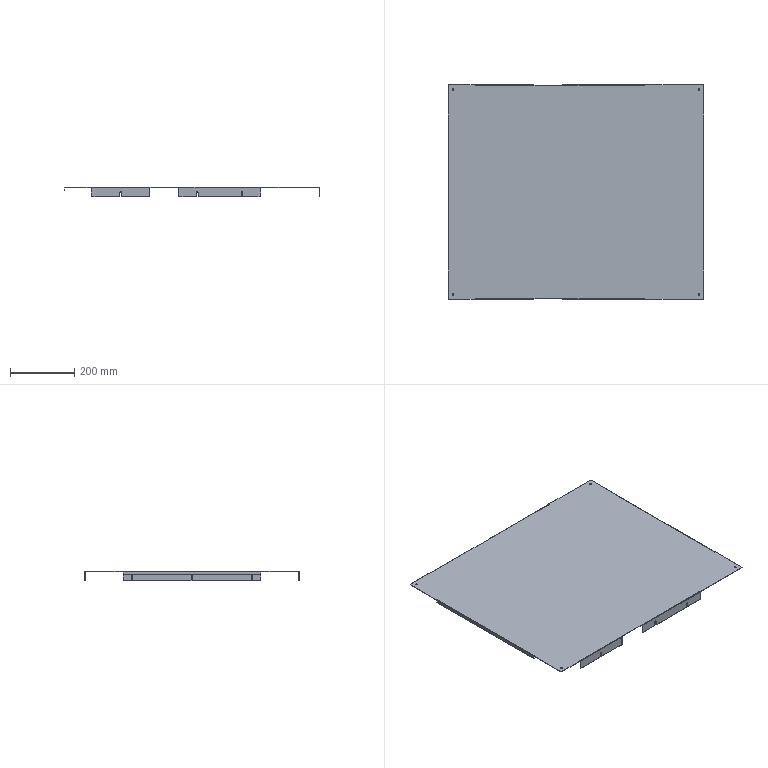Part | STEP file | 1 solid | 161 faces | box 798 x 668 x 30 mm | volume 686782 mm3 | plane 109 | cylinder 52 | commonest cylinder face diameters 4.5 x18 4 x14 5 x8 1.2 x6 3.6 x6